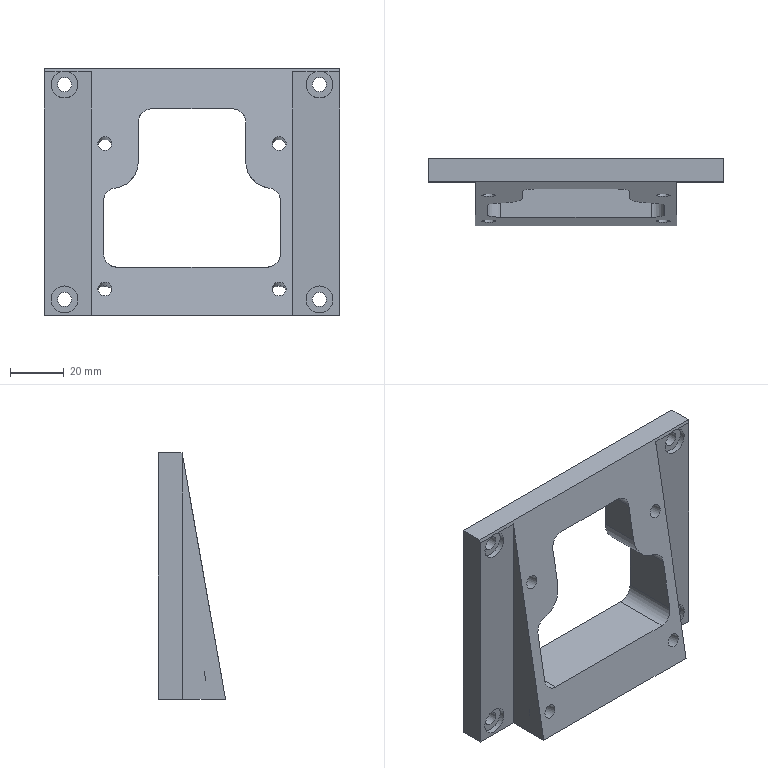NC program | NX | posted by the shop | part box 110 x 25 x 92 mm
Whole program, first 1079 of 1169 lines:
%
O0001
(Machine time: 3.08 MIN)
(===Total Tool:4===)
(T6=D6      D=6.   R=0.   D-  H06 Z=-18.52)
(T7=D6-J    D=6.   R=0.   D7  H07 Z=-18.62)
(T2=D6 chamfer cutter   D=6.   R=0.   D-  H02 Z=-19.42)
(T17=ZT5.2  D=5.2  DR_a=118 D-  H17 Z=-28.18)
G80 G90 G17 G49 G40
G91 G28 Z0
M01
N1 T06 M06
(D6  D=6. R=0. H=06 ce=0.06 di=0.10)
G00 G90 G54 X-83.111 Y31.886 M03 S8000
G43 H06 Z50.
M08
Z.884
G01 X-83.004 Y32.158 Z.869 F1500.
Y32.5 Z.851
Y32.842 Z.833
X-83.298 Y33.583 Z.791
X-83.861 Y34.146 Z.749
X-84.601 Y34.44 Z.707
X-84.944 Z.689
X-85.286 Z.671
X-86.026 Y34.146 Z.63
X-86.589 Y33.583 Z.588
X-86.884 Y32.842 Z.546
Y32.158 Z.51
X-86.589 Y31.417 Z.469
X-86.026 Y30.854 Z.427
X-85.286 Y30.56 Z.385
X-84.944 Z.367
X-84.601 Z.349
X-83.861 Y30.854 Z.308
X-83.298 Y31.417 Z.266
X-83.004 Y32.158 Z.224
Y32.5 Z.206
Y32.842 Z.188
X-83.298 Y33.583 Z.146
X-83.861 Y34.146 Z.105
X-84.601 Y34.44 Z.063
X-84.944 Z.045
X-85.286 Z.027
X-86.026 Y34.146 Z-.015
X-86.589 Y33.583 Z-.056
X-86.884 Y32.842 Z-.098
Y32.5 Z-.116
G03 X-84.944 Y30.56 Z-.19 I1.94 J0.0
X-83.004 Y32.5 Z-.265 I0.0 J1.94
X-84.944 Y34.44 Z-.339 I-1.94 J0.0
X-86.884 Y32.5 Z-.413 I0.0 J-1.94
X-84.944 Y30.56 Z-.487 I1.94 J0.0
X-83.004 Y32.5 Z-.561 I0.0 J1.94
X-84.944 Y34.44 Z-.636 I-1.94 J0.0
X-86.884 Y32.5 Z-.71 I0.0 J-1.94
X-84.944 Y30.56 Z-.784 I1.94 J0.0
X-83.004 Y32.5 Z-.858 I0.0 J1.94
X-84.944 Y34.44 Z-.932 I-1.94 J0.0
X-86.884 Y32.5 Z-1.007 I0.0 J-1.94
X-84.944 Y30.56 Z-1.081 I1.94 J0.0
X-83.004 Y32.5 Z-1.155 I0.0 J1.94
X-84.944 Y34.44 Z-1.229 I-1.94 J0.0
X-86.884 Y32.5 Z-1.304 I0.0 J-1.94
X-84.944 Y30.56 Z-1.378 I1.94 J0.0
X-83.004 Y32.5 Z-1.452 I0.0 J1.94
X-84.944 Y34.44 Z-1.526 I-1.94 J0.0
X-86.884 Y32.5 Z-1.6 I0.0 J-1.94
X-84.944 Y30.56 Z-1.675 I1.94 J0.0
X-83.004 Y32.5 Z-1.749 I0.0 J1.94
X-84.944 Y34.44 Z-1.823 I-1.94 J0.0
X-86.884 Y32.5 Z-1.897 I0.0 J-1.94
X-84.944 Y30.56 Z-1.971 I1.94 J0.0
X-83.004 Y32.5 Z-2.046 I0.0 J1.94
X-84.944 Y34.44 Z-2.12 I-1.94 J0.0
X-86.884 Y32.5 Z-2.194 I0.0 J-1.94
X-84.944 Y30.56 Z-2.268 I1.94 J0.0
X-83.004 Y32.5 Z-2.342 I0.0 J1.94
X-84.944 Y34.44 Z-2.417 I-1.94 J0.0
X-86.884 Y32.5 Z-2.491 I0.0 J-1.94
X-84.944 Y30.56 Z-2.565 I1.94 J0.0
X-83.004 Y32.5 Z-2.639 I0.0 J1.94
X-84.944 Y34.44 Z-2.714 I-1.94 J0.0
X-86.884 Y32.5 Z-2.788 I0.0 J-1.94
X-84.944 Y30.56 Z-2.862 I1.94 J0.0
X-83.004 Y32.5 Z-2.936 I0.0 J1.94
X-84.944 Y34.44 Z-3.01 I-1.94 J0.0
X-86.884 Y32.5 Z-3.085 I0.0 J-1.94
X-84.944 Y30.56 Z-3.159 I1.94 J0.0
X-83.004 Y32.5 Z-3.233 I0.0 J1.94
X-84.944 Y34.44 Z-3.307 I-1.94 J0.0
X-86.884 Y32.5 Z-3.381 I0.0 J-1.94
X-84.944 Y30.56 Z-3.456 I1.94 J0.0
X-83.004 Y32.5 Z-3.53 I0.0 J1.94
X-84.944 Y34.44 Z-3.604 I-1.94 J0.0
X-86.884 Y32.5 Z-3.678 I0.0 J-1.94
X-84.944 Y30.56 Z-3.752 I1.94 J0.0
X-83.004 Y32.5 Z-3.827 I0.0 J1.94
X-84.944 Y34.44 Z-3.901 I-1.94 J0.0
X-86.884 Y32.5 Z-3.975 I0.0 J-1.94
X-84.944 Y30.56 Z-4.049 I1.94 J0.0
X-83.004 Y32.5 Z-4.123 I0.0 J1.94
X-84.944 Y34.44 Z-4.198 I-1.94 J0.0
X-86.884 Y32.5 Z-4.272 I0.0 J-1.94
X-84.944 Y30.56 Z-4.346 I1.94 J0.0
X-83.004 Y32.5 Z-4.42 I0.0 J1.94
X-84.944 Y34.44 Z-4.495 I-1.94 J0.0
X-86.884 Y32.5 Z-4.569 I0.0 J-1.94
X-84.944 Y30.56 Z-4.643 I1.94 J0.0
X-83.004 Y32.5 Z-4.717 I0.0 J1.94
X-84.944 Y34.44 Z-4.791 I-1.94 J0.0
X-86.884 Y32.5 Z-4.866 I0.0 J-1.94
X-84.944 Y30.56 Z-4.94 I1.94 J0.0
X-83.004 Y32.5 Z-5.014 I0.0 J1.94
X-84.944 Y34.44 Z-5.088 I-1.94 J0.0
X-86.884 Y32.5 Z-5.162 I0.0 J-1.94
X-84.944 Y30.56 Z-5.237 I1.94 J0.0
X-83.004 Y32.5 Z-5.311 I0.0 J1.94
X-84.944 Y34.44 Z-5.385 I-1.94 J0.0
X-86.884 Y32.5 Z-5.459 I0.0 J-1.94
X-84.944 Y30.56 Z-5.533 I1.94 J0.0
X-83.004 Y32.5 Z-5.608 I0.0 J1.94
X-84.944 Y34.44 Z-5.682 I-1.94 J0.0
X-86.884 Y32.5 Z-5.756 I0.0 J-1.94
X-84.944 Y30.56 Z-5.83 I1.94 J0.0
X-83.004 Y32.5 Z-5.905 I0.0 J1.94
X-84.944 Y34.44 Z-5.979 I-1.94 J0.0
X-86.884 Y32.5 Z-6.053 I0.0 J-1.94
X-84.944 Y30.56 Z-6.127 I1.94 J0.0
X-83.004 Y32.5 Z-6.201 I0.0 J1.94
X-84.944 Y34.44 Z-6.276 I-1.94 J0.0
X-86.884 Y32.5 Z-6.35 I0.0 J-1.94
X-84.944 Y30.56 Z-6.424 I1.94 J0.0
X-83.004 Y32.5 Z-6.498 I0.0 J1.94
X-84.944 Y34.44 Z-6.572 I-1.94 J0.0
X-86.884 Y32.5 Z-6.647 I0.0 J-1.94
X-84.944 Y30.56 Z-6.721 I1.94 J0.0
X-83.004 Y32.5 Z-6.795 I0.0 J1.94
X-84.944 Y34.44 Z-6.869 I-1.94 J0.0
X-86.884 Y32.5 Z-6.943 I0.0 J-1.94
X-84.944 Y30.56 Z-7.018 I1.94 J0.0
X-83.004 Y32.5 Z-7.092 I0.0 J1.94
X-84.944 Y34.44 Z-7.166 I-1.94 J0.0
X-86.884 Y32.5 Z-7.24 I0.0 J-1.94
X-84.944 Y30.56 Z-7.315 I1.94 J0.0
X-83.004 Y32.5 Z-7.389 I0.0 J1.94
X-84.944 Y34.44 Z-7.463 I-1.94 J0.0
X-86.884 Y32.5 Z-7.537 I0.0 J-1.94
X-84.944 Y30.56 Z-7.611 I1.94 J0.0
X-83.004 Y32.5 Z-7.686 I0.0 J1.94
X-84.944 Y34.44 Z-7.76 I-1.94 J0.0
X-86.884 Y32.5 Z-7.834 I0.0 J-1.94
X-84.944 Y30.56 Z-7.908 I1.94 J0.0
X-83.004 Y32.5 Z-7.982 I0.0 J1.94
X-84.944 Y34.44 Z-8.057 I-1.94 J0.0
X-86.884 Y32.5 Z-8.131 I0.0 J-1.94
X-84.944 Y30.56 Z-8.205 I1.94 J0.0
X-83.004 Y32.5 Z-8.279 I0.0 J1.94
X-84.944 Y34.44 Z-8.353 I-1.94 J0.0
X-86.884 Y32.5 Z-8.428 I0.0 J-1.94
X-84.944 Y30.56 Z-8.502 I1.94 J0.0
X-83.004 Y32.5 Z-8.576 I0.0 J1.94
X-84.944 Y34.44 Z-8.65 I-1.94 J0.0
X-86.884 Y32.5 Z-8.725 I0.0 J-1.94
X-84.944 Y30.56 Z-8.799 I1.94 J0.0
X-83.004 Y32.5 Z-8.873 I0.0 J1.94
X-84.944 Y34.44 Z-8.947 I-1.94 J0.0
X-86.884 Y32.5 Z-9.021 I0.0 J-1.94
X-84.944 Y30.56 Z-9.096 I1.94 J0.0
X-83.004 Y32.5 Z-9.17 I0.0 J1.94
X-84.944 Y34.44 Z-9.244 I-1.94 J0.0
X-86.884 Y32.5 Z-9.318 I0.0 J-1.94
X-84.944 Y30.56 Z-9.392 I1.94 J0.0
X-83.004 Y32.5 Z-9.467 I0.0 J1.94
X-84.944 Y34.44 Z-9.541 I-1.94 J0.0
X-86.884 Y32.5 Z-9.615 I0.0 J-1.94
X-84.944 Y30.56 Z-9.689 I1.94 J0.0
X-83.004 Y32.5 Z-9.763 I0.0 J1.94
X-84.944 Y34.44 Z-9.838 I-1.94 J0.0
X-86.884 Y32.5 Z-9.912 I0.0 J-1.94
X-84.944 Y30.56 Z-9.986 I1.94 J0.0
X-83.004 Y32.5 Z-10.06 I0.0 J1.94
X-84.944 Y34.44 Z-10.134 I-1.94 J0.0
X-86.884 Y32.5 Z-10.209 I0.0 J-1.94
X-84.944 Y30.56 Z-10.283 I1.94 J0.0
X-83.004 Y32.5 Z-10.357 I0.0 J1.94
X-84.944 Y34.44 Z-10.431 I-1.94 J0.0
X-86.884 Y32.5 Z-10.506 I0.0 J-1.94
X-84.944 Y30.56 Z-10.58 I1.94 J0.0
X-83.004 Y32.5 Z-10.654 I0.0 J1.94
X-84.944 Y34.44 Z-10.728 I-1.94 J0.0
X-86.884 Y32.5 Z-10.802 I0.0 J-1.94
X-84.944 Y30.56 Z-10.877 I1.94 J0.0
X-83.004 Y32.5 Z-10.951 I0.0 J1.94
X-84.944 Y34.44 Z-11.025 I-1.94 J0.0
X-86.884 Y32.5 Z-11.099 I0.0 J-1.94
X-84.944 Y30.56 Z-11.173 I1.94 J0.0
X-83.004 Y32.5 Z-11.248 I0.0 J1.94
X-84.944 Y34.44 Z-11.322 I-1.94 J0.0
X-86.884 Y32.5 Z-11.396 I0.0 J-1.94
X-84.944 Y30.56 Z-11.47 I1.94 J0.0
X-83.004 Y32.5 Z-11.544 I0.0 J1.94
X-84.944 Y34.44 Z-11.619 I-1.94 J0.0
X-86.884 Y32.5 Z-11.693 I0.0 J-1.94
X-84.944 Y30.56 Z-11.767 I1.94 J0.0
X-83.004 Y32.5 Z-11.841 I0.0 J1.94
X-84.944 Y34.44 Z-11.916 I-1.94 J0.0
X-86.884 Y32.5 Z-11.99 I0.0 J-1.94
X-84.944 Y30.56 Z-12.064 I1.94 J0.0
X-83.004 Y32.5 Z-12.138 I0.0 J1.94
X-84.944 Y34.44 Z-12.212 I-1.94 J0.0
X-86.884 Y32.5 Z-12.287 I0.0 J-1.94
X-84.944 Y30.56 Z-12.361 I1.94 J0.0
X-83.004 Y32.5 Z-12.435 I0.0 J1.94
X-84.944 Y34.44 Z-12.509 I-1.94 J0.0
X-86.884 Y32.5 Z-12.583 I0.0 J-1.94
X-84.944 Y30.56 Z-12.658 I1.94 J0.0
X-83.004 Y32.5 Z-12.732 I0.0 J1.94
X-84.944 Y34.44 Z-12.806 I-1.94 J0.0
X-86.884 Y32.5 Z-12.88 I0.0 J-1.94
X-84.944 Y30.56 Z-12.954 I1.94 J0.0
X-83.004 Y32.5 Z-13.029 I0.0 J1.94
X-84.944 Y34.44 Z-13.103 I-1.94 J0.0
X-86.884 Y32.5 Z-13.177 I0.0 J-1.94
X-84.944 Y30.56 Z-13.251 I1.94 J0.0
X-83.004 Y32.5 Z-13.326 I0.0 J1.94
X-84.944 Y34.44 Z-13.4 I-1.94 J0.0
X-86.884 Y32.5 Z-13.474 I0.0 J-1.94
X-84.944 Y30.56 Z-13.548 I1.94 J0.0
X-83.004 Y32.5 Z-13.622 I0.0 J1.94
X-84.944 Y34.44 Z-13.697 I-1.94 J0.0
X-86.884 Y32.5 Z-13.771 I0.0 J-1.94
X-84.944 Y30.56 Z-13.845 I1.94 J0.0
X-83.004 Y32.5 Z-13.919 I0.0 J1.94
X-84.944 Y34.44 Z-13.993 I-1.94 J0.0
X-86.884 Y32.5 Z-14.068 I0.0 J-1.94
X-84.944 Y30.56 Z-14.142 I1.94 J0.0
X-83.004 Y32.5 Z-14.216 I0.0 J1.94
X-84.944 Y34.44 Z-14.29 I-1.94 J0.0
X-86.884 Y32.5 Z-14.364 I0.0 J-1.94
X-84.944 Y30.56 Z-14.439 I1.94 J0.0
X-83.004 Y32.5 Z-14.513 I0.0 J1.94
X-84.944 Y34.44 Z-14.587 I-1.94 J0.0
X-86.884 Y32.5 Z-14.661 I0.0 J-1.94
X-84.944 Y30.56 Z-14.735 I1.94 J0.0
X-83.004 Y32.5 Z-14.81 I0.0 J1.94
X-84.944 Y34.44 Z-14.884 I-1.94 J0.0
X-86.884 Y32.5 Z-14.958 I0.0 J-1.94
X-84.944 Y30.56 Z-15.032 I1.94 J0.0
X-83.004 Y32.5 Z-15.107 I0.0 J1.94
X-84.944 Y34.44 Z-15.181 I-1.94 J0.0
X-86.884 Y32.5 Z-15.255 I0.0 J-1.94
X-84.944 Y30.56 Z-15.329 I1.94 J0.0
X-83.004 Y32.5 Z-15.403 I0.0 J1.94
X-84.944 Y34.44 Z-15.478 I-1.94 J0.0
X-86.884 Y32.5 Z-15.552 I0.0 J-1.94
X-84.944 Y30.56 Z-15.626 I1.94 J0.0
X-83.004 Y32.5 Z-15.7 I0.0 J1.94
X-84.944 Y34.44 Z-15.774 I-1.94 J0.0
X-86.884 Y32.5 Z-15.849 I0.0 J-1.94
X-84.944 Y30.56 Z-15.923 I1.94 J0.0
X-83.004 Y32.5 Z-15.997 I0.0 J1.94
X-84.944 Y34.44 Z-16.071 I-1.94 J0.0
X-86.884 Y32.5 Z-16.145 I0.0 J-1.94
X-84.944 Y30.56 Z-16.22 I1.94 J0.0
X-83.004 Y32.5 Z-16.294 I0.0 J1.94
X-84.944 Y34.44 Z-16.368 I-1.94 J0.0
X-86.884 Y32.5 Z-16.442 I0.0 J-1.94
X-84.944 Y30.56 Z-16.517 I1.94 J0.0
X-83.004 Y32.5 Z-16.591 I0.0 J1.94
X-84.944 Y34.44 Z-16.665 I-1.94 J0.0
X-86.884 Y32.5 Z-16.739 I0.0 J-1.94
X-84.944 Y30.56 Z-16.813 I1.94 J0.0
X-83.004 Y32.5 Z-16.888 I0.0 J1.94
X-84.944 Y34.44 Z-16.962 I-1.94 J0.0
X-86.884 Y32.5 Z-17.036 I0.0 J-1.94
X-84.944 Y30.56 Z-17.11 I1.94 J0.0
X-83.004 Y32.5 Z-17.184 I0.0 J1.94
X-84.944 Y34.44 Z-17.259 I-1.94 J0.0
X-86.884 Y32.5 Z-17.333 I0.0 J-1.94
X-84.944 Y30.56 Z-17.407 I1.94 J0.0
X-83.004 Y32.5 Z-17.481 I0.0 J1.94
X-84.944 Y34.44 Z-17.555 I-1.94 J0.0
X-86.884 Y32.5 Z-17.63 I0.0 J-1.94
X-84.944 Y30.56 Z-17.704 I1.94 J0.0
X-83.004 Y32.5 Z-17.778 I0.0 J1.94
X-84.944 Y34.44 Z-17.852 I-1.94 J0.0
X-86.884 Y32.5 Z-17.927 I0.0 J-1.94
X-84.944 Y30.56 Z-18.001 I1.94 J0.0
X-83.004 Y32.5 Z-18.075 I0.0 J1.94
X-84.944 Y34.44 Z-18.149 I-1.94 J0.0
X-86.884 Y32.5 Z-18.223 I0.0 J-1.94
X-84.944 Y30.56 Z-18.298 I1.94 J0.0
X-83.004 Y32.5 Z-18.372 I0.0 J1.94
X-84.944 Y34.44 Z-18.446 I-1.94 J0.0
X-86.884 Y32.5 Z-18.52 I0.0 J-1.94
X-84.944 Y30.56 I1.94 J0.0
X-83.004 Y32.5 I0.0 J1.94
X-84.944 Y34.44 I-1.94 J0.0
X-86.884 Y32.5 I0.0 J-1.94
X-86.842 Y32.103 I1.94 J0.0
G01 Z-17.52
G00 Z50.
X-30.558 Y30.668
Z-8.814
G01 X-30.286 Y30.56 Z-8.829
X-29.601 Z-8.865
X-28.861 Y30.854 Z-8.907
X-28.298 Y31.417 Z-8.949
X-28.004 Y32.158 Z-8.991
Y32.842 Z-9.026
X-28.298 Y33.583 Z-9.068
X-28.861 Y34.146 Z-9.11
X-29.601 Y34.44 Z-9.152
X-30.286 Z-9.188
X-31.026 Y34.146 Z-9.229
X-31.589 Y33.583 Z-9.271
X-31.884 Y32.842 Z-9.313
Y32.158 Z-9.349
X-31.589 Y31.417 Z-9.39
X-31.026 Y30.854 Z-9.432
X-30.286 Y30.56 Z-9.474
X-29.601 Z-9.51
X-28.861 Y30.854 Z-9.552
X-28.298 Y31.417 Z-9.593
X-28.004 Y32.158 Z-9.635
Y32.842 Z-9.671
X-28.298 Y33.583 Z-9.713
X-28.861 Y34.146 Z-9.754
X-29.601 Y34.44 Z-9.796
X-29.944 Z-9.814
G03 X-31.884 Y32.5 Z-9.887 I0.0 J-1.94
X-29.944 Y30.56 Z-9.959 I1.94 J0.0
X-28.004 Y32.5 Z-10.032 I0.0 J1.94
X-29.944 Y34.44 Z-10.104 I-1.94 J0.0
X-31.884 Y32.5 Z-10.177 I0.0 J-1.94
X-29.944 Y30.56 Z-10.249 I1.94 J0.0
X-28.004 Y32.5 Z-10.322 I0.0 J1.94
X-29.944 Y34.44 Z-10.395 I-1.94 J0.0
X-31.884 Y32.5 Z-10.467 I0.0 J-1.94
X-29.944 Y30.56 Z-10.54 I1.94 J0.0
X-28.004 Y32.5 Z-10.612 I0.0 J1.94
X-29.944 Y34.44 Z-10.685 I-1.94 J0.0
X-31.884 Y32.5 Z-10.757 I0.0 J-1.94
X-29.944 Y30.56 Z-10.83 I1.94 J0.0
X-28.004 Y32.5 Z-10.902 I0.0 J1.94
X-29.944 Y34.44 Z-10.975 I-1.94 J0.0
X-31.884 Y32.5 Z-11.048 I0.0 J-1.94
X-29.944 Y30.56 Z-11.12 I1.94 J0.0
X-28.004 Y32.5 Z-11.193 I0.0 J1.94
X-29.944 Y34.44 Z-11.265 I-1.94 J0.0
X-31.884 Y32.5 Z-11.338 I0.0 J-1.94
X-29.944 Y30.56 Z-11.41 I1.94 J0.0
X-28.004 Y32.5 Z-11.483 I0.0 J1.94
X-29.944 Y34.44 Z-11.555 I-1.94 J0.0
X-31.884 Y32.5 Z-11.628 I0.0 J-1.94
X-29.944 Y30.56 Z-11.7 I1.94 J0.0
X-28.004 Y32.5 Z-11.773 I0.0 J1.94
X-29.944 Y34.44 Z-11.846 I-1.94 J0.0
X-31.884 Y32.5 Z-11.918 I0.0 J-1.94
X-29.944 Y30.56 Z-11.991 I1.94 J0.0
X-28.004 Y32.5 Z-12.063 I0.0 J1.94
X-29.944 Y34.44 Z-12.136 I-1.94 J0.0
X-31.884 Y32.5 Z-12.208 I0.0 J-1.94
X-29.944 Y30.56 Z-12.281 I1.94 J0.0
X-28.004 Y32.5 Z-12.353 I0.0 J1.94
X-29.944 Y34.44 Z-12.426 I-1.94 J0.0
X-31.884 Y32.5 Z-12.499 I0.0 J-1.94
X-29.944 Y30.56 Z-12.571 I1.94 J0.0
X-28.004 Y32.5 Z-12.644 I0.0 J1.94
X-29.944 Y34.44 Z-12.716 I-1.94 J0.0
X-31.884 Y32.5 Z-12.789 I0.0 J-1.94
X-29.944 Y30.56 Z-12.861 I1.94 J0.0
X-28.004 Y32.5 Z-12.934 I0.0 J1.94
X-29.944 Y34.44 Z-13.006 I-1.94 J0.0
X-31.884 Y32.5 Z-13.079 I0.0 J-1.94
X-29.944 Y30.56 Z-13.151 I1.94 J0.0
X-28.004 Y32.5 Z-13.224 I0.0 J1.94
X-29.944 Y34.44 Z-13.297 I-1.94 J0.0
X-31.884 Y32.5 Z-13.369 I0.0 J-1.94
X-29.944 Y30.56 Z-13.442 I1.94 J0.0
X-28.004 Y32.5 Z-13.514 I0.0 J1.94
X-29.944 Y34.44 Z-13.587 I-1.94 J0.0
X-31.884 Y32.5 Z-13.659 I0.0 J-1.94
X-29.944 Y30.56 Z-13.732 I1.94 J0.0
X-28.004 Y32.5 Z-13.804 I0.0 J1.94
X-29.944 Y34.44 Z-13.877 I-1.94 J0.0
X-31.884 Y32.5 Z-13.95 I0.0 J-1.94
X-29.944 Y30.56 Z-14.022 I1.94 J0.0
X-28.004 Y32.5 Z-14.095 I0.0 J1.94
X-29.944 Y34.44 Z-14.167 I-1.94 J0.0
X-31.884 Y32.5 Z-14.24 I0.0 J-1.94
X-29.944 Y30.56 Z-14.312 I1.94 J0.0
X-28.004 Y32.5 Z-14.385 I0.0 J1.94
X-29.944 Y34.44 Z-14.457 I-1.94 J0.0
X-31.884 Y32.5 Z-14.53 I0.0 J-1.94
X-29.944 Y30.56 Z-14.602 I1.94 J0.0
X-28.004 Y32.5 Z-14.675 I0.0 J1.94
X-29.944 Y34.44 Z-14.748 I-1.94 J0.0
X-31.884 Y32.5 Z-14.82 I0.0 J-1.94
X-29.944 Y30.56 Z-14.893 I1.94 J0.0
X-28.004 Y32.5 Z-14.965 I0.0 J1.94
X-29.944 Y34.44 Z-15.038 I-1.94 J0.0
X-31.884 Y32.5 Z-15.11 I0.0 J-1.94
X-29.944 Y30.56 Z-15.183 I1.94 J0.0
X-28.004 Y32.5 Z-15.255 I0.0 J1.94
X-29.944 Y34.44 Z-15.328 I-1.94 J0.0
X-31.884 Y32.5 Z-15.401 I0.0 J-1.94
X-29.944 Y30.56 Z-15.473 I1.94 J0.0
X-28.004 Y32.5 Z-15.546 I0.0 J1.94
X-29.944 Y34.44 Z-15.618 I-1.94 J0.0
X-31.884 Y32.5 Z-15.691 I0.0 J-1.94
X-29.944 Y30.56 Z-15.763 I1.94 J0.0
X-28.004 Y32.5 Z-15.836 I0.0 J1.94
X-29.944 Y34.44 Z-15.908 I-1.94 J0.0
X-31.884 Y32.5 Z-15.981 I0.0 J-1.94
X-29.944 Y30.56 Z-16.053 I1.94 J0.0
X-28.004 Y32.5 Z-16.126 I0.0 J1.94
X-29.944 Y34.44 Z-16.199 I-1.94 J0.0
X-31.884 Y32.5 Z-16.271 I0.0 J-1.94
X-29.944 Y30.56 Z-16.344 I1.94 J0.0
X-28.004 Y32.5 Z-16.416 I0.0 J1.94
X-29.944 Y34.44 Z-16.489 I-1.94 J0.0
X-31.884 Y32.5 Z-16.561 I0.0 J-1.94
X-29.944 Y30.56 Z-16.634 I1.94 J0.0
X-28.004 Y32.5 Z-16.706 I0.0 J1.94
X-29.944 Y34.44 Z-16.779 I-1.94 J0.0
X-31.884 Y32.5 Z-16.852 I0.0 J-1.94
X-29.944 Y30.56 Z-16.924 I1.94 J0.0
X-28.004 Y32.5 Z-16.997 I0.0 J1.94
X-29.944 Y34.44 Z-17.069 I-1.94 J0.0
X-31.884 Y32.5 Z-17.142 I0.0 J-1.94
X-29.944 Y30.56 Z-17.214 I1.94 J0.0
X-28.004 Y32.5 Z-17.287 I0.0 J1.94
X-29.944 Y34.44 Z-17.359 I-1.94 J0.0
X-31.884 Y32.5 Z-17.432 I0.0 J-1.94
X-29.944 Y30.56 Z-17.504 I1.94 J0.0
X-28.004 Y32.5 Z-17.577 I0.0 J1.94
X-29.944 Y34.44 Z-17.65 I-1.94 J0.0
X-31.884 Y32.5 Z-17.722 I0.0 J-1.94
X-29.944 Y30.56 Z-17.795 I1.94 J0.0
X-28.004 Y32.5 Z-17.867 I0.0 J1.94
X-29.944 Y34.44 Z-17.94 I-1.94 J0.0
X-31.884 Y32.5 Z-18.012 I0.0 J-1.94
X-29.944 Y30.56 Z-18.085 I1.94 J0.0
X-28.004 Y32.5 Z-18.157 I0.0 J1.94
X-29.944 Y34.44 Z-18.23 I-1.94 J0.0
X-31.884 Y32.5 Z-18.303 I0.0 J-1.94
X-29.944 Y30.56 Z-18.375 I1.94 J0.0
X-28.004 Y32.5 Z-18.448 I0.0 J1.94
X-29.944 Y34.44 Z-18.52 I-1.94 J0.0
X-31.884 Y32.5 I0.0 J-1.94
X-29.944 Y30.56 I1.94 J0.0
X-28.004 Y32.5 I0.0 J1.94
X-29.944 Y34.44 I-1.94 J0.0
X-30.341 Y34.399 I0.0 J-1.94
G01 Z-17.52
G00 Z50.
X-29.329 Y-30.668
Z-8.814
G01 X-29.601 Y-30.56 Z-8.829
X-30.286 Z-8.865
X-31.026 Y-30.854 Z-8.907
X-31.589 Y-31.417 Z-8.949
X-31.884 Y-32.158 Z-8.991
Y-32.842 Z-9.026
X-31.589 Y-33.583 Z-9.068
X-31.026 Y-34.146 Z-9.11
X-30.286 Y-34.44 Z-9.152
X-29.601 Z-9.188
X-28.861 Y-34.146 Z-9.229
X-28.298 Y-33.583 Z-9.271
X-28.004 Y-32.842 Z-9.313
Y-32.158 Z-9.349
X-28.298 Y-31.417 Z-9.39
X-28.861 Y-30.854 Z-9.432
X-29.601 Y-30.56 Z-9.474
X-30.286 Z-9.51
X-31.026 Y-30.854 Z-9.552
X-31.589 Y-31.417 Z-9.593
X-31.884 Y-32.158 Z-9.635
Y-32.842 Z-9.671
X-31.589 Y-33.583 Z-9.713
X-31.026 Y-34.146 Z-9.754
X-30.286 Y-34.44 Z-9.796
X-29.944 Z-9.814
G03 X-28.004 Y-32.5 Z-9.887 I0.0 J1.94
X-29.944 Y-30.56 Z-9.959 I-1.94 J0.0
X-31.884 Y-32.5 Z-10.032 I0.0 J-1.94
X-29.944 Y-34.44 Z-10.104 I1.94 J0.0
X-28.004 Y-32.5 Z-10.177 I0.0 J1.94
X-29.944 Y-30.56 Z-10.249 I-1.94 J0.0
X-31.884 Y-32.5 Z-10.322 I0.0 J-1.94
X-29.944 Y-34.44 Z-10.395 I1.94 J0.0
X-28.004 Y-32.5 Z-10.467 I0.0 J1.94
X-29.944 Y-30.56 Z-10.54 I-1.94 J0.0
X-31.884 Y-32.5 Z-10.612 I0.0 J-1.94
X-29.944 Y-34.44 Z-10.685 I1.94 J0.0
X-28.004 Y-32.5 Z-10.757 I0.0 J1.94
X-29.944 Y-30.56 Z-10.83 I-1.94 J0.0
X-31.884 Y-32.5 Z-10.902 I0.0 J-1.94
X-29.944 Y-34.44 Z-10.975 I1.94 J0.0
X-28.004 Y-32.5 Z-11.048 I0.0 J1.94
X-29.944 Y-30.56 Z-11.12 I-1.94 J0.0
X-31.884 Y-32.5 Z-11.193 I0.0 J-1.94
X-29.944 Y-34.44 Z-11.265 I1.94 J0.0
X-28.004 Y-32.5 Z-11.338 I0.0 J1.94
X-29.944 Y-30.56 Z-11.41 I-1.94 J0.0
X-31.884 Y-32.5 Z-11.483 I0.0 J-1.94
X-29.944 Y-34.44 Z-11.555 I1.94 J0.0
X-28.004 Y-32.5 Z-11.628 I0.0 J1.94
X-29.944 Y-30.56 Z-11.7 I-1.94 J0.0
X-31.884 Y-32.5 Z-11.773 I0.0 J-1.94
X-29.944 Y-34.44 Z-11.846 I1.94 J0.0
X-28.004 Y-32.5 Z-11.918 I0.0 J1.94
X-29.944 Y-30.56 Z-11.991 I-1.94 J0.0
X-31.884 Y-32.5 Z-12.063 I0.0 J-1.94
X-29.944 Y-34.44 Z-12.136 I1.94 J0.0
X-28.004 Y-32.5 Z-12.208 I0.0 J1.94
X-29.944 Y-30.56 Z-12.281 I-1.94 J0.0
X-31.884 Y-32.5 Z-12.353 I0.0 J-1.94
X-29.944 Y-34.44 Z-12.426 I1.94 J0.0
X-28.004 Y-32.5 Z-12.499 I0.0 J1.94
X-29.944 Y-30.56 Z-12.571 I-1.94 J0.0
X-31.884 Y-32.5 Z-12.644 I0.0 J-1.94
X-29.944 Y-34.44 Z-12.716 I1.94 J0.0
X-28.004 Y-32.5 Z-12.789 I0.0 J1.94
X-29.944 Y-30.56 Z-12.861 I-1.94 J0.0
X-31.884 Y-32.5 Z-12.934 I0.0 J-1.94
X-29.944 Y-34.44 Z-13.006 I1.94 J0.0
X-28.004 Y-32.5 Z-13.079 I0.0 J1.94
X-29.944 Y-30.56 Z-13.151 I-1.94 J0.0
X-31.884 Y-32.5 Z-13.224 I0.0 J-1.94
X-29.944 Y-34.44 Z-13.297 I1.94 J0.0
X-28.004 Y-32.5 Z-13.369 I0.0 J1.94
X-29.944 Y-30.56 Z-13.442 I-1.94 J0.0
X-31.884 Y-32.5 Z-13.514 I0.0 J-1.94
X-29.944 Y-34.44 Z-13.587 I1.94 J0.0
X-28.004 Y-32.5 Z-13.659 I0.0 J1.94
X-29.944 Y-30.56 Z-13.732 I-1.94 J0.0
X-31.884 Y-32.5 Z-13.804 I0.0 J-1.94
X-29.944 Y-34.44 Z-13.877 I1.94 J0.0
X-28.004 Y-32.5 Z-13.95 I0.0 J1.94
X-29.944 Y-30.56 Z-14.022 I-1.94 J0.0
X-31.884 Y-32.5 Z-14.095 I0.0 J-1.94
X-29.944 Y-34.44 Z-14.167 I1.94 J0.0
X-28.004 Y-32.5 Z-14.24 I0.0 J1.94
X-29.944 Y-30.56 Z-14.312 I-1.94 J0.0
X-31.884 Y-32.5 Z-14.385 I0.0 J-1.94
X-29.944 Y-34.44 Z-14.457 I1.94 J0.0
X-28.004 Y-32.5 Z-14.53 I0.0 J1.94
X-29.944 Y-30.56 Z-14.602 I-1.94 J0.0
X-31.884 Y-32.5 Z-14.675 I0.0 J-1.94
X-29.944 Y-34.44 Z-14.748 I1.94 J0.0
X-28.004 Y-32.5 Z-14.82 I0.0 J1.94
X-29.944 Y-30.56 Z-14.893 I-1.94 J0.0
X-31.884 Y-32.5 Z-14.965 I0.0 J-1.94
X-29.944 Y-34.44 Z-15.038 I1.94 J0.0
X-28.004 Y-32.5 Z-15.11 I0.0 J1.94
X-29.944 Y-30.56 Z-15.183 I-1.94 J0.0
X-31.884 Y-32.5 Z-15.255 I0.0 J-1.94
X-29.944 Y-34.44 Z-15.328 I1.94 J0.0
X-28.004 Y-32.5 Z-15.401 I0.0 J1.94
X-29.944 Y-30.56 Z-15.473 I-1.94 J0.0
X-31.884 Y-32.5 Z-15.546 I0.0 J-1.94
X-29.944 Y-34.44 Z-15.618 I1.94 J0.0
X-28.004 Y-32.5 Z-15.691 I0.0 J1.94
X-29.944 Y-30.56 Z-15.763 I-1.94 J0.0
X-31.884 Y-32.5 Z-15.836 I0.0 J-1.94
X-29.944 Y-34.44 Z-15.908 I1.94 J0.0
X-28.004 Y-32.5 Z-15.981 I0.0 J1.94
X-29.944 Y-30.56 Z-16.053 I-1.94 J0.0
X-31.884 Y-32.5 Z-16.126 I0.0 J-1.94
X-29.944 Y-34.44 Z-16.199 I1.94 J0.0
X-28.004 Y-32.5 Z-16.271 I0.0 J1.94
X-29.944 Y-30.56 Z-16.344 I-1.94 J0.0
X-31.884 Y-32.5 Z-16.416 I0.0 J-1.94
X-29.944 Y-34.44 Z-16.489 I1.94 J0.0
X-28.004 Y-32.5 Z-16.561 I0.0 J1.94
X-29.944 Y-30.56 Z-16.634 I-1.94 J0.0
X-31.884 Y-32.5 Z-16.706 I0.0 J-1.94
X-29.944 Y-34.44 Z-16.779 I1.94 J0.0
X-28.004 Y-32.5 Z-16.852 I0.0 J1.94
X-29.944 Y-30.56 Z-16.924 I-1.94 J0.0
X-31.884 Y-32.5 Z-16.997 I0.0 J-1.94
X-29.944 Y-34.44 Z-17.069 I1.94 J0.0
X-28.004 Y-32.5 Z-17.142 I0.0 J1.94
X-29.944 Y-30.56 Z-17.214 I-1.94 J0.0
X-31.884 Y-32.5 Z-17.287 I0.0 J-1.94
X-29.944 Y-34.44 Z-17.359 I1.94 J0.0
X-28.004 Y-32.5 Z-17.432 I0.0 J1.94
X-29.944 Y-30.56 Z-17.504 I-1.94 J0.0
X-31.884 Y-32.5 Z-17.577 I0.0 J-1.94
X-29.944 Y-34.44 Z-17.65 I1.94 J0.0
X-28.004 Y-32.5 Z-17.722 I0.0 J1.94
X-29.944 Y-30.56 Z-17.795 I-1.94 J0.0
X-31.884 Y-32.5 Z-17.867 I0.0 J-1.94
X-29.944 Y-34.44 Z-17.94 I1.94 J0.0
X-28.004 Y-32.5 Z-18.012 I0.0 J1.94
X-29.944 Y-30.56 Z-18.085 I-1.94 J0.0
X-31.884 Y-32.5 Z-18.157 I0.0 J-1.94
X-29.944 Y-34.44 Z-18.23 I1.94 J0.0
X-28.004 Y-32.5 Z-18.303 I0.0 J1.94
X-29.944 Y-30.56 Z-18.375 I-1.94 J0.0
X-31.884 Y-32.5 Z-18.448 I0.0 J-1.94
X-29.944 Y-34.44 Z-18.52 I1.94 J0.0
X-28.004 Y-32.5 I0.0 J1.94
X-29.944 Y-30.56 I-1.94 J0.0
X-31.884 Y-32.5 I0.0 J-1.94
X-29.944 Y-34.44 I1.94 J0.0
X-29.546 Y-34.399 I0.0 J1.94
G01 Z-17.52
G00 Z50.
X-83.111 Y-33.114
Z.884
G01 X-83.004 Y-32.842 Z.869
Y-32.5 Z.851
Y-32.158 Z.833
X-83.298 Y-31.417 Z.791
X-83.861 Y-30.854 Z.749
X-84.601 Y-30.56 Z.707
X-84.944 Z.689
X-85.286 Z.671
X-86.026 Y-30.854 Z.63
X-86.589 Y-31.417 Z.588
X-86.884 Y-32.158 Z.546
Y-32.5 Z.528
Y-32.842 Z.51
X-86.589 Y-33.583 Z.469
X-86.026 Y-34.146 Z.427
X-85.286 Y-34.44 Z.385
X-84.944 Z.367
X-84.601 Z.349
X-83.861 Y-34.146 Z.308
X-83.298 Y-33.583 Z.266
X-83.004 Y-32.842 Z.224
Y-32.5 Z.206
Y-32.158 Z.188
X-83.298 Y-31.417 Z.146
X-83.861 Y-30.854 Z.105
X-84.601 Y-30.56 Z.063
X-84.944 Z.045
X-85.286 Z.027
X-86.026 Y-30.854 Z-.015
X-86.589 Y-31.417 Z-.056
X-86.884 Y-32.158 Z-.098
Y-32.5 Z-.116
G03 X-84.944 Y-34.44 Z-.19 I1.94 J0.0
X-83.004 Y-32.5 Z-.265 I0.0 J1.94
X-84.944 Y-30.56 Z-.339 I-1.94 J0.0
X-86.884 Y-32.5 Z-.413 I0.0 J-1.94
X-84.944 Y-34.44 Z-.487 I1.94 J0.0
X-83.004 Y-32.5 Z-.561 I0.0 J1.94
X-84.944 Y-30.56 Z-.636 I-1.94 J0.0
X-86.884 Y-32.5 Z-.71 I0.0 J-1.94
X-84.944 Y-34.44 Z-.784 I1.94 J0.0
X-83.004 Y-32.5 Z-.858 I0.0 J1.94
X-84.944 Y-30.56 Z-.932 I-1.94 J0.0
X-86.884 Y-32.5 Z-1.007 I0.0 J-1.94
X-84.944 Y-34.44 Z-1.081 I1.94 J0.0
X-83.004 Y-32.5 Z-1.155 I0.0 J1.94
X-84.944 Y-30.56 Z-1.229 I-1.94 J0.0
X-86.884 Y-32.5 Z-1.304 I0.0 J-1.94
X-84.944 Y-34.44 Z-1.378 I1.94 J0.0
X-83.004 Y-32.5 Z-1.452 I0.0 J1.94
X-84.944 Y-30.56 Z-1.526 I-1.94 J0.0
X-86.884 Y-32.5 Z-1.6 I0.0 J-1.94
X-84.944 Y-34.44 Z-1.675 I1.94 J0.0
X-83.004 Y-32.5 Z-1.749 I0.0 J1.94
X-84.944 Y-30.56 Z-1.823 I-1.94 J0.0
X-86.884 Y-32.5 Z-1.897 I0.0 J-1.94
X-84.944 Y-34.44 Z-1.971 I1.94 J0.0
X-83.004 Y-32.5 Z-2.046 I0.0 J1.94
X-84.944 Y-30.56 Z-2.12 I-1.94 J0.0
X-86.884 Y-32.5 Z-2.194 I0.0 J-1.94
X-84.944 Y-34.44 Z-2.268 I1.94 J0.0
X-83.004 Y-32.5 Z-2.342 I0.0 J1.94
X-84.944 Y-30.56 Z-2.417 I-1.94 J0.0
X-86.884 Y-32.5 Z-2.491 I0.0 J-1.94
X-84.944 Y-34.44 Z-2.565 I1.94 J0.0
X-83.004 Y-32.5 Z-2.639 I0.0 J1.94
X-84.944 Y-30.56 Z-2.714 I-1.94 J0.0
X-86.884 Y-32.5 Z-2.788 I0.0 J-1.94
X-84.944 Y-34.44 Z-2.862 I1.94 J0.0
X-83.004 Y-32.5 Z-2.936 I0.0 J1.94
X-84.944 Y-30.56 Z-3.01 I-1.94 J0.0
X-86.884 Y-32.5 Z-3.085 I0.0 J-1.94
X-84.944 Y-34.44 Z-3.159 I1.94 J0.0
X-83.004 Y-32.5 Z-3.233 I0.0 J1.94
X-84.944 Y-30.56 Z-3.307 I-1.94 J0.0
X-86.884 Y-32.5 Z-3.381 I0.0 J-1.94
X-84.944 Y-34.44 Z-3.456 I1.94 J0.0
X-83.004 Y-32.5 Z-3.53 I0.0 J1.94
X-84.944 Y-30.56 Z-3.604 I-1.94 J0.0
X-86.884 Y-32.5 Z-3.678 I0.0 J-1.94
X-84.944 Y-34.44 Z-3.752 I1.94 J0.0
X-83.004 Y-32.5 Z-3.827 I0.0 J1.94
X-84.944 Y-30.56 Z-3.901 I-1.94 J0.0
X-86.884 Y-32.5 Z-3.975 I0.0 J-1.94
X-84.944 Y-34.44 Z-4.049 I1.94 J0.0
X-83.004 Y-32.5 Z-4.123 I0.0 J1.94
X-84.944 Y-30.56 Z-4.198 I-1.94 J0.0
X-86.884 Y-32.5 Z-4.272 I0.0 J-1.94
X-84.944 Y-34.44 Z-4.346 I1.94 J0.0
X-83.004 Y-32.5 Z-4.42 I0.0 J1.94
X-84.944 Y-30.56 Z-4.495 I-1.94 J0.0
X-86.884 Y-32.5 Z-4.569 I0.0 J-1.94
X-84.944 Y-34.44 Z-4.643 I1.94 J0.0
X-83.004 Y-32.5 Z-4.717 I0.0 J1.94
X-84.944 Y-30.56 Z-4.791 I-1.94 J0.0
X-86.884 Y-32.5 Z-4.866 I0.0 J-1.94
X-84.944 Y-34.44 Z-4.94 I1.94 J0.0
X-83.004 Y-32.5 Z-5.014 I0.0 J1.94
X-84.944 Y-30.56 Z-5.088 I-1.94 J0.0
X-86.884 Y-32.5 Z-5.162 I0.0 J-1.94
X-84.944 Y-34.44 Z-5.237 I1.94 J0.0
X-83.004 Y-32.5 Z-5.311 I0.0 J1.94
X-84.944 Y-30.56 Z-5.385 I-1.94 J0.0
X-86.884 Y-32.5 Z-5.459 I0.0 J-1.94
X-84.944 Y-34.44 Z-5.533 I1.94 J0.0
X-83.004 Y-32.5 Z-5.608 I0.0 J1.94
X-84.944 Y-30.56 Z-5.682 I-1.94 J0.0
X-86.884 Y-32.5 Z-5.756 I0.0 J-1.94
X-84.944 Y-34.44 Z-5.83 I1.94 J0.0
X-83.004 Y-32.5 Z-5.905 I0.0 J1.94
X-84.944 Y-30.56 Z-5.979 I-1.94 J0.0
X-86.884 Y-32.5 Z-6.053 I0.0 J-1.94
X-84.944 Y-34.44 Z-6.127 I1.94 J0.0
X-83.004 Y-32.5 Z-6.201 I0.0 J1.94
X-84.944 Y-30.56 Z-6.276 I-1.94 J0.0
X-86.884 Y-32.5 Z-6.35 I0.0 J-1.94
X-84.944 Y-34.44 Z-6.424 I1.94 J0.0
X-83.004 Y-32.5 Z-6.498 I0.0 J1.94
X-84.944 Y-30.56 Z-6.572 I-1.94 J0.0
X-86.884 Y-32.5 Z-6.647 I0.0 J-1.94
X-84.944 Y-34.44 Z-6.721 I1.94 J0.0
X-83.004 Y-32.5 Z-6.795 I0.0 J1.94
X-84.944 Y-30.56 Z-6.869 I-1.94 J0.0
X-86.884 Y-32.5 Z-6.943 I0.0 J-1.94
X-84.944 Y-34.44 Z-7.018 I1.94 J0.0
X-83.004 Y-32.5 Z-7.092 I0.0 J1.94
X-84.944 Y-30.56 Z-7.166 I-1.94 J0.0
X-86.884 Y-32.5 Z-7.24 I0.0 J-1.94
X-84.944 Y-34.44 Z-7.315 I1.94 J0.0
X-83.004 Y-32.5 Z-7.389 I0.0 J1.94
X-84.944 Y-30.56 Z-7.463 I-1.94 J0.0
X-86.884 Y-32.5 Z-7.537 I0.0 J-1.94
X-84.944 Y-34.44 Z-7.611 I1.94 J0.0
X-83.004 Y-32.5 Z-7.686 I0.0 J1.94
X-84.944 Y-30.56 Z-7.76 I-1.94 J0.0
X-86.884 Y-32.5 Z-7.834 I0.0 J-1.94
X-84.944 Y-34.44 Z-7.908 I1.94 J0.0
X-83.004 Y-32.5 Z-7.982 I0.0 J1.94
X-84.944 Y-30.56 Z-8.057 I-1.94 J0.0
X-86.884 Y-32.5 Z-8.131 I0.0 J-1.94
X-84.944 Y-34.44 Z-8.205 I1.94 J0.0
X-83.004 Y-32.5 Z-8.279 I0.0 J1.94
X-84.944 Y-30.56 Z-8.353 I-1.94 J0.0
X-86.884 Y-32.5 Z-8.428 I0.0 J-1.94
X-84.944 Y-34.44 Z-8.502 I1.94 J0.0
X-83.004 Y-32.5 Z-8.576 I0.0 J1.94
X-84.944 Y-30.56 Z-8.65 I-1.94 J0.0
X-86.884 Y-32.5 Z-8.725 I0.0 J-1.94
X-84.944 Y-34.44 Z-8.799 I1.94 J0.0
X-83.004 Y-32.5 Z-8.873 I0.0 J1.94
X-84.944 Y-30.56 Z-8.947 I-1.94 J0.0
X-86.884 Y-32.5 Z-9.021 I0.0 J-1.94
X-84.944 Y-34.44 Z-9.096 I1.94 J0.0
X-83.004 Y-32.5 Z-9.17 I0.0 J1.94
X-84.944 Y-30.56 Z-9.244 I-1.94 J0.0
X-86.884 Y-32.5 Z-9.318 I0.0 J-1.94
X-84.944 Y-34.44 Z-9.392 I1.94 J0.0
X-83.004 Y-32.5 Z-9.467 I0.0 J1.94
X-84.944 Y-30.56 Z-9.541 I-1.94 J0.0
X-86.884 Y-32.5 Z-9.615 I0.0 J-1.94
X-84.944 Y-34.44 Z-9.689 I1.94 J0.0
X-83.004 Y-32.5 Z-9.763 I0.0 J1.94
X-84.944 Y-30.56 Z-9.838 I-1.94 J0.0
X-86.884 Y-32.5 Z-9.912 I0.0 J-1.94
X-84.944 Y-34.44 Z-9.986 I1.94 J0.0
X-83.004 Y-32.5 Z-10.06 I0.0 J1.94
X-84.944 Y-30.56 Z-10.134 I-1.94 J0.0
X-86.884 Y-32.5 Z-10.209 I0.0 J-1.94
X-84.944 Y-34.44 Z-10.283 I1.94 J0.0
X-83.004 Y-32.5 Z-10.357 I0.0 J1.94
X-84.944 Y-30.56 Z-10.431 I-1.94 J0.0
X-86.884 Y-32.5 Z-10.506 I0.0 J-1.94
X-84.944 Y-34.44 Z-10.58 I1.94 J0.0
X-83.004 Y-32.5 Z-10.654 I0.0 J1.94
X-84.944 Y-30.56 Z-10.728 I-1.94 J0.0
X-86.884 Y-32.5 Z-10.802 I0.0 J-1.94
X-84.944 Y-34.44 Z-10.877 I1.94 J0.0
X-83.004 Y-32.5 Z-10.951 I0.0 J1.94
X-84.944 Y-30.56 Z-11.025 I-1.94 J0.0
X-86.884 Y-32.5 Z-11.099 I0.0 J-1.94
X-84.944 Y-34.44 Z-11.173 I1.94 J0.0
X-83.004 Y-32.5 Z-11.248 I0.0 J1.94
X-84.944 Y-30.56 Z-11.322 I-1.94 J0.0
X-86.884 Y-32.5 Z-11.396 I0.0 J-1.94
X-84.944 Y-34.44 Z-11.47 I1.94 J0.0
X-83.004 Y-32.5 Z-11.544 I0.0 J1.94
X-84.944 Y-30.56 Z-11.619 I-1.94 J0.0
X-86.884 Y-32.5 Z-11.693 I0.0 J-1.94
X-84.944 Y-34.44 Z-11.767 I1.94 J0.0
X-83.004 Y-32.5 Z-11.841 I0.0 J1.94
X-84.944 Y-30.56 Z-11.916 I-1.94 J0.0
X-86.884 Y-32.5 Z-11.99 I0.0 J-1.94
X-84.944 Y-34.44 Z-12.064 I1.94 J0.0
X-83.004 Y-32.5 Z-12.138 I0.0 J1.94
X-84.944 Y-30.56 Z-12.212 I-1.94 J0.0
X-86.884 Y-32.5 Z-12.287 I0.0 J-1.94
X-84.944 Y-34.44 Z-12.361 I1.94 J0.0
X-83.004 Y-32.5 Z-12.435 I0.0 J1.94
X-84.944 Y-30.56 Z-12.509 I-1.94 J0.0
X-86.884 Y-32.5 Z-12.583 I0.0 J-1.94
X-84.944 Y-34.44 Z-12.658 I1.94 J0.0
X-83.004 Y-32.5 Z-12.732 I0.0 J1.94
X-84.944 Y-30.56 Z-12.806 I-1.94 J0.0
X-86.884 Y-32.5 Z-12.88 I0.0 J-1.94
X-84.944 Y-34.44 Z-12.954 I1.94 J0.0
X-83.004 Y-32.5 Z-13.029 I0.0 J1.94
X-84.944 Y-30.56 Z-13.103 I-1.94 J0.0
X-86.884 Y-32.5 Z-13.177 I0.0 J-1.94
X-84.944 Y-34.44 Z-13.251 I1.94 J0.0
X-83.004 Y-32.5 Z-13.326 I0.0 J1.94
X-84.944 Y-30.56 Z-13.4 I-1.94 J0.0
X-86.884 Y-32.5 Z-13.474 I0.0 J-1.94
X-84.944 Y-34.44 Z-13.548 I1.94 J0.0
X-83.004 Y-32.5 Z-13.622 I0.0 J1.94
X-84.944 Y-30.56 Z-13.697 I-1.94 J0.0
X-86.884 Y-32.5 Z-13.771 I0.0 J-1.94
X-84.944 Y-34.44 Z-13.845 I1.94 J0.0
X-83.004 Y-32.5 Z-13.919 I0.0 J1.94
X-84.944 Y-30.56 Z-13.993 I-1.94 J0.0
X-86.884 Y-32.5 Z-14.068 I0.0 J-1.94
X-84.944 Y-34.44 Z-14.142 I1.94 J0.0
X-83.004 Y-32.5 Z-14.216 I0.0 J1.94
X-84.944 Y-30.56 Z-14.29 I-1.94 J0.0
X-86.884 Y-32.5 Z-14.364 I0.0 J-1.94
X-84.944 Y-34.44 Z-14.439 I1.94 J0.0
X-83.004 Y-32.5 Z-14.513 I0.0 J1.94
X-84.944 Y-30.56 Z-14.587 I-1.94 J0.0
X-86.884 Y-32.5 Z-14.661 I0.0 J-1.94
X-84.944 Y-34.44 Z-14.735 I1.94 J0.0
X-83.004 Y-32.5 Z-14.81 I0.0 J1.94
X-84.944 Y-30.56 Z-14.884 I-1.94 J0.0
X-86.884 Y-32.5 Z-14.958 I0.0 J-1.94
X-84.944 Y-34.44 Z-15.032 I1.94 J0.0
X-83.004 Y-32.5 Z-15.107 I0.0 J1.94
X-84.944 Y-30.56 Z-15.181 I-1.94 J0.0
X-86.884 Y-32.5 Z-15.255 I0.0 J-1.94
X-84.944 Y-34.44 Z-15.329 I1.94 J0.0
X-83.004 Y-32.5 Z-15.403 I0.0 J1.94
X-84.944 Y-30.56 Z-15.478 I-1.94 J0.0
X-86.884 Y-32.5 Z-15.552 I0.0 J-1.94
X-84.944 Y-34.44 Z-15.626 I1.94 J0.0
X-83.004 Y-32.5 Z-15.7 I0.0 J1.94
X-84.944 Y-30.56 Z-15.774 I-1.94 J0.0
X-86.884 Y-32.5 Z-15.849 I0.0 J-1.94
X-84.944 Y-34.44 Z-15.923 I1.94 J0.0
X-83.004 Y-32.5 Z-15.997 I0.0 J1.94
X-84.944 Y-30.56 Z-16.071 I-1.94 J0.0
X-86.884 Y-32.5 Z-16.145 I0.0 J-1.94
X-84.944 Y-34.44 Z-16.22 I1.94 J0.0
X-83.004 Y-32.5 Z-16.294 I0.0 J1.94
X-84.944 Y-30.56 Z-16.368 I-1.94 J0.0
X-86.884 Y-32.5 Z-16.442 I0.0 J-1.94
X-84.944 Y-34.44 Z-16.517 I1.94 J0.0
X-83.004 Y-32.5 Z-16.591 I0.0 J1.94
X-84.944 Y-30.56 Z-16.665 I-1.94 J0.0
X-86.884 Y-32.5 Z-16.739 I0.0 J-1.94
X-84.944 Y-34.44 Z-16.813 I1.94 J0.0
X-83.004 Y-32.5 Z-16.888 I0.0 J1.94
X-84.944 Y-30.56 Z-16.962 I-1.94 J0.0
X-86.884 Y-32.5 Z-17.036 I0.0 J-1.94
X-84.944 Y-34.44 Z-17.11 I1.94 J0.0
X-83.004 Y-32.5 Z-17.184 I0.0 J1.94
X-84.944 Y-30.56 Z-17.259 I-1.94 J0.0
X-86.884 Y-32.5 Z-17.333 I0.0 J-1.94
X-84.944 Y-34.44 Z-17.407 I1.94 J0.0
X-83.004 Y-32.5 Z-17.481 I0.0 J1.94
X-84.944 Y-30.56 Z-17.555 I-1.94 J0.0
X-86.884 Y-32.5 Z-17.63 I0.0 J-1.94
X-84.944 Y-34.44 Z-17.704 I1.94 J0.0
X-83.004 Y-32.5 Z-17.778 I0.0 J1.94
X-84.944 Y-30.56 Z-17.852 I-1.94 J0.0
X-86.884 Y-32.5 Z-17.927 I0.0 J-1.94
X-84.944 Y-34.44 Z-18.001 I1.94 J0.0
X-83.004 Y-32.5 Z-18.075 I0.0 J1.94
X-84.944 Y-30.56 Z-18.149 I-1.94 J0.0
X-86.884 Y-32.5 Z-18.223 I0.0 J-1.94
X-84.944 Y-34.44 Z-18.298 I1.94 J0.0
X-83.004 Y-32.5 Z-18.372 I0.0 J1.94
X-84.944 Y-30.56 Z-18.446 I-1.94 J0.0
X-86.884 Y-32.5 Z-18.52 I0.0 J-1.94
X-84.944 Y-34.44 I1.94 J0.0
X-83.004 Y-32.5 I0.0 J1.94
X-84.944 Y-30.56 I-1.94 J0.0
X-86.884 Y-32.5 I0.0 J-1.94
X-86.842 Y-32.897 I1.94 J0.0
G01 Z-17.52
G00 Z50.
G91 G28 Z0.0
M05
M09
G91 G28 Z0.0
M01
N2 T07 M06
(D6-J  D=6. R=0. H=07 ce=0.00 di=0.00)
G00 G90 G54 X-85.247 Y30.561 M03 S8000
G43 H07 Z50.
M08
Z.384
G01 X-85.084 Y30.535 Z.375 F1000.
X-84.803 Z.36
X-84.457 Y30.591 Z.342
X-84.125 Y30.708 Z.324
X-83.82 Y30.882 Z.305
X-83.551 Y31.107 Z.287
X-83.325 Y31.377 Z.268
X-83.152 Y31.682 Z.25
X-83.035 Y32.013 Z.232
X-82.979 Y32.36 Z.213
Y32.64 Z.199
X-83.035 Y32.987 Z.18
X-83.152 Y33.318 Z.162
X-83.325 Y33.623 Z.143
X-83.551 Y33.893 Z.125
X-83.82 Y34.118 Z.106
X-84.125 Y34.292 Z.088
X-84.457 Y34.409 Z.07
X-84.803 Y34.465 Z.051
X-85.084 Z.037
X-85.474 Y34.397 Z.016
X-85.843 Y34.253 Z-.005
X-86.176 Y34.037 Z-.026
X-86.458 Y33.76 Z-.047
X-86.68 Y33.431 Z-.067
X-86.831 Y33.065 Z-.088
X-86.906 Y32.676 Z-.109
X-86.908 Y32.535 Z-.116
G41 D07
X-86.944 Y32.5
G03 X-84.944 Y30.5 Z-1.273 I2. J0.0
X-82.944 Y32.5 Z-2.429 I0.0 J2.
X-84.944 Y34.5 Z-3.586 I-2. J0.0
X-86.944 Y32.5 Z-4.742 I0.0 J-2.
X-84.944 Y30.5 Z-5.899 I2. J0.0
X-82.944 Y32.5 Z-7.055 I0.0 J2.
X-84.944 Y34.5 Z-8.212 I-2. J0.0
X-86.944 Y32.5 Z-9.368 I0.0 J-2.
X-84.944 Y30.5 Z-10.525 I2. J0.0
X-82.944 Y32.5 Z-11.681 I0.0 J2.
X-84.944 Y34.5 Z-12.838 I-2. J0.0
X-86.944 Y32.5 Z-13.994 I0.0 J-2.
X-84.944 Y30.5 Z-15.151 I2. J0.0
X-82.944 Y32.5 Z-16.307 I0.0 J2.
X-84.944 Y34.5 Z-17.464 I-2. J0.0
X-86.944 Y32.5 Z-18.62 I0.0 J-2.
X-84.944 Y30.5 I2. J0.0
X-82.944 Y32.5 I0.0 J2.
X-84.944 Y34.5 I-2. J0.0
X-86.944 Y32.5 I0.0 J-2.
X-86.904 Y32.103 I2. J0.0
G01 X-86.896 Y32.076
X-86.872 Y32.06
X-86.845 Y32.064
G40 X-86.796 Y32.074
Z-17.62
G00 Z50.
X-31.882 Y32.804
Z-9.314
G01 X-31.908 Y32.64 Z-9.323
Y32.36 Z-9.338
X-31.852 Y32.013 Z-9.356
X-31.736 Y31.682 Z-9.374
X-31.562 Y31.377 Z-9.393
X-31.336 Y31.107 Z-9.411
X-31.067 Y30.882 Z-9.43
X-30.762 Y30.708 Z-9.448
X-30.431 Y30.591 Z-9.466
X-30.084 Y30.535 Z-9.485
X-29.803 Z-9.499
X-29.457 Y30.591 Z-9.518
X-29.125 Y30.708 Z-9.536
X-28.82 Y30.882 Z-9.555
X-28.551 Y31.107 Z-9.573
X-28.325 Y31.377 Z-9.592
X-28.152 Y31.682 Z-9.61
X-28.035 Y32.013 Z-9.628
X-27.979 Y32.36 Z-9.647
Y32.64 Z-9.661
X-28.046 Y33.031 Z-9.682
X-28.191 Y33.4 Z-9.703
X-28.406 Y33.732 Z-9.724
X-28.684 Y34.015 Z-9.745
X-29.013 Y34.236 Z-9.765
X-29.379 Y34.387 Z-9.786
X-29.768 Y34.462 Z-9.807
X-29.908 Y34.465 Z-9.814
G41 D07
X-29.944 Y34.5
G03 X-31.944 Y32.5 Z-10.915 I0.0 J-2.
X-29.944 Y30.5 Z-12.016 I2. J0.0
X-27.944 Y32.5 Z-13.116 I0.0 J2.
X-29.944 Y34.5 Z-14.217 I-2. J0.0
X-31.944 Y32.5 Z-15.318 I0.0 J-2.
X-29.944 Y30.5 Z-16.419 I2. J0.0
X-27.944 Y32.5 Z-17.519 I0.0 J2.
X-29.944 Y34.5 Z-18.62 I-2. J0.0
X-31.944 Y32.5 I0.0 J-2.
X-29.944 Y30.5 I2. J0.0
X-27.944 Y32.5 I0.0 J2.
X-29.944 Y34.5 I-2. J0.0
X-30.341 Y34.46 I0.0 J-2.
G01 X-30.367 Y34.452
X-30.383 Y34.429
X-30.38 Y34.401
G40 X-30.37 Y34.352
Z-17.62
G00 Z50.
X-28.005 Y-32.804
Z-9.314
G01 X-27.979 Y-32.64 Z-9.323
Y-32.36 Z-9.338
X-28.035 Y-32.013 Z-9.356
X-28.152 Y-31.682 Z-9.374
X-28.325 Y-31.377 Z-9.393
X-28.551 Y-31.107 Z-9.411
X-28.82 Y-30.882 Z-9.43
X-29.125 Y-30.708 Z-9.448
X-29.457 Y-30.591 Z-9.466
X-29.803 Y-30.535 Z-9.485
X-30.084 Z-9.499
X-30.431 Y-30.591 Z-9.518
X-30.762 Y-30.708 Z-9.536
X-31.067 Y-30.882 Z-9.555
X-31.336 Y-31.107 Z-9.573
X-31.562 Y-31.377 Z-9.592
X-31.736 Y-31.682 Z-9.61
X-31.852 Y-32.013 Z-9.628
X-31.908 Y-32.36 Z-9.647
Y-32.64 Z-9.661
X-31.841 Y-33.031 Z-9.682
X-31.696 Y-33.4 Z-9.703
X-31.481 Y-33.732 Z-9.724
X-31.203 Y-34.015 Z-9.745
X-30.874 Y-34.236 Z-9.765
X-30.508 Y-34.387 Z-9.786
X-30.119 Y-34.462 Z-9.807
X-29.979 Y-34.465 Z-9.814
G41 D07
X-29.944 Y-34.5
G03 X-27.944 Y-32.5 Z-10.915 I0.0 J2.
X-29.944 Y-30.5 Z-12.016 I-2. J0.0
X-31.944 Y-32.5 Z-13.116 I0.0 J-2.
X-29.944 Y-34.5 Z-14.217 I2. J0.0
X-27.944 Y-32.5 Z-15.318 I0.0 J2.
X-29.944 Y-30.5 Z-16.419 I-2. J0.0
X-31.944 Y-32.5 Z-17.519 I0.0 J-2.
X-29.944 Y-34.5 Z-18.62 I2. J0.0
X-27.944 Y-32.5 I0.0 J2.
X-29.944 Y-30.5 I-2. J0.0
X-31.944 Y-32.5 I0.0 J-2.
X-29.944 Y-34.5 I2. J0.0
X-29.546 Y-34.46 I0.0 J2.
G01 X-29.52 Y-34.452
X-29.504 Y-34.429
X-29.507 Y-34.401
G40 X-29.517 Y-34.352
Z-17.62
G00 Z50.
X-85.247 Y-34.439
Z.384
G01 X-85.084 Y-34.465 Z.375
X-84.803 Z.36
X-84.457 Y-34.409 Z.342
X-84.125 Y-34.292 Z.324
X-83.82 Y-34.118 Z.305